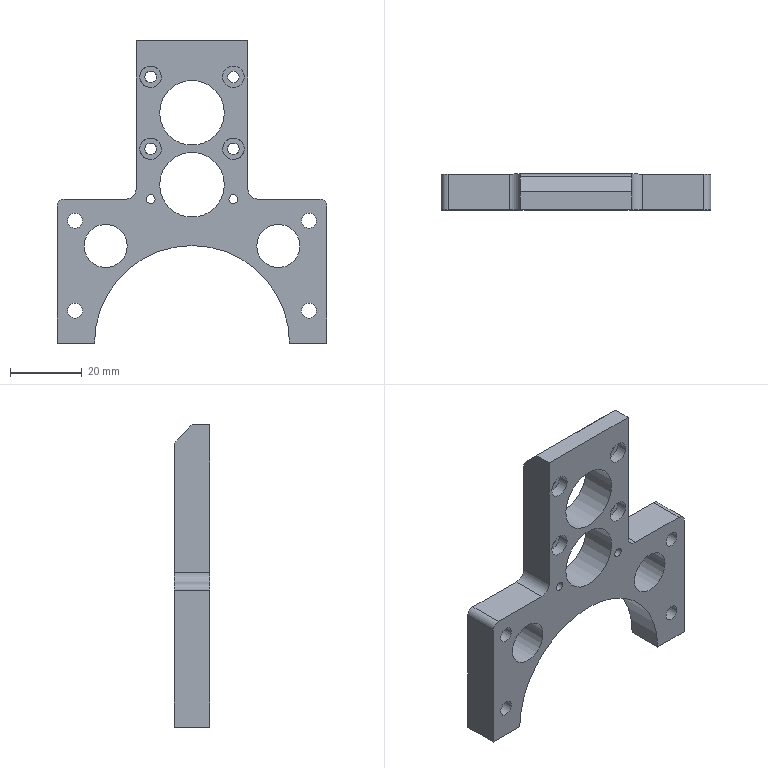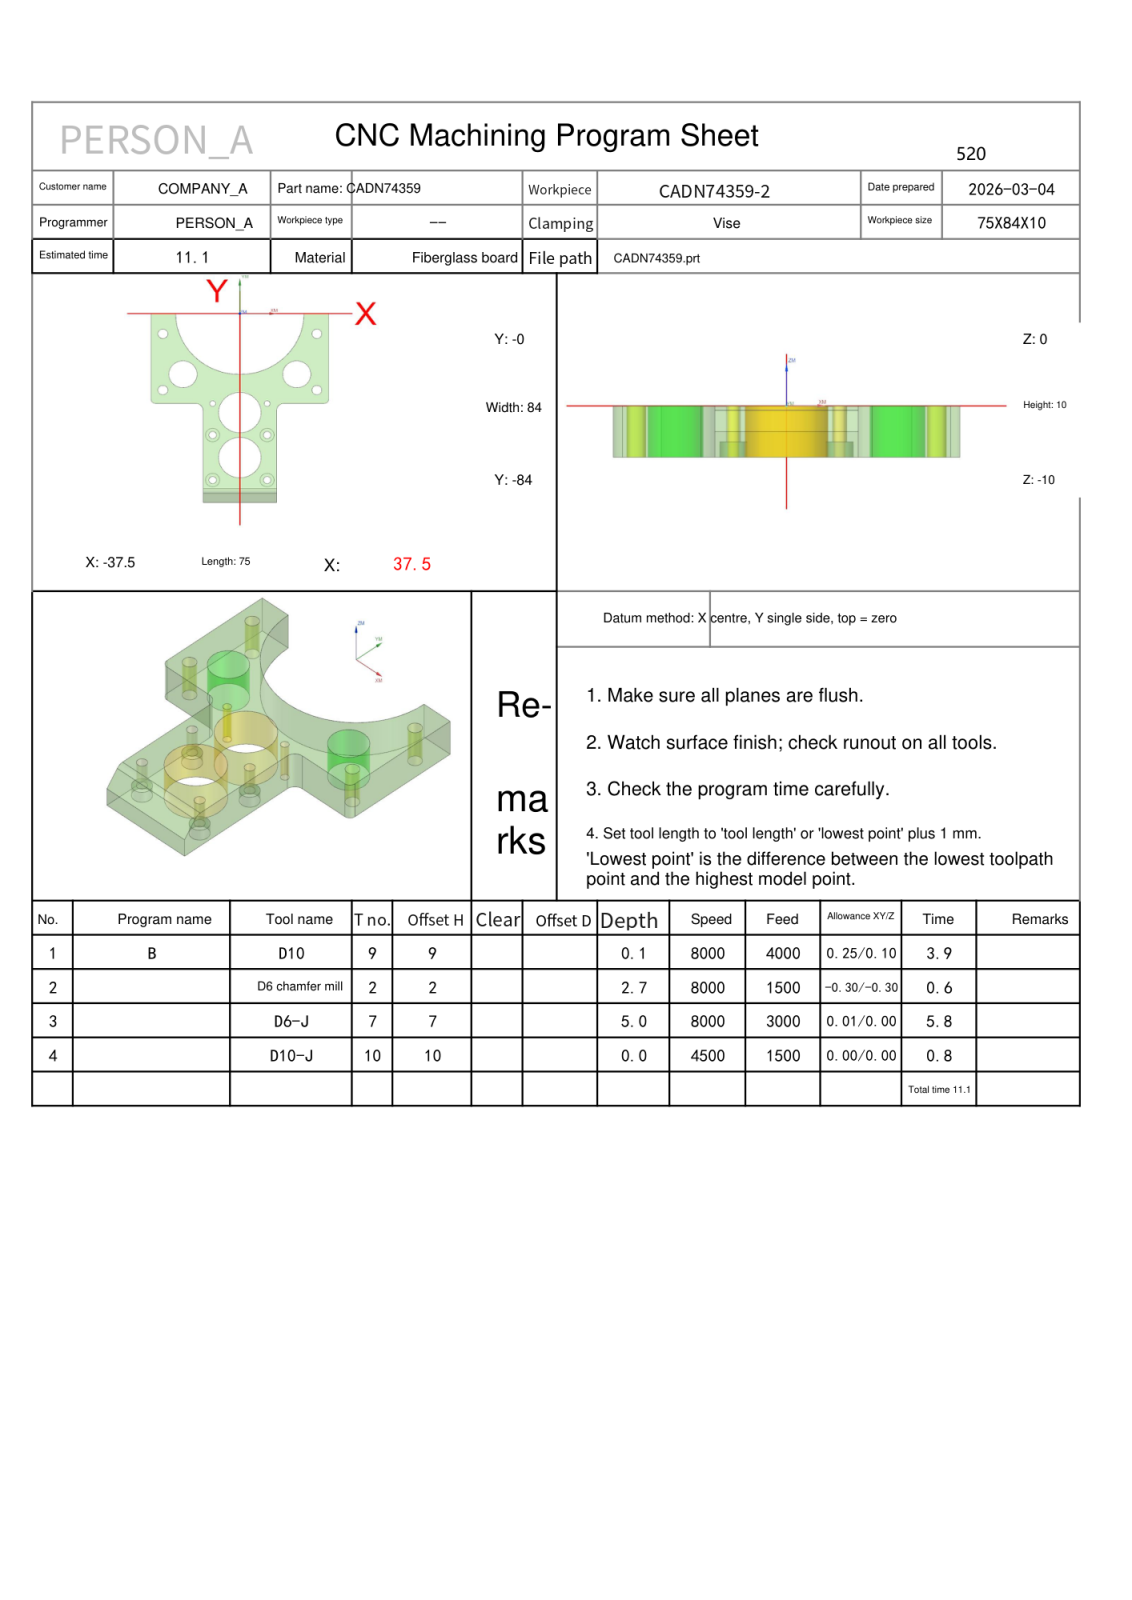NC program | NX | posted by the shop | part box 75 x 10 x 84 mm
Lines 5662 to 5701 of 5701:
N4 T10 M06
(D10-J  D=10. R=0. H=10 ce=0.00 di=0.00)
G00 G90 G54 X-35.962 Y-94. M03 S4500
G43 H10 Z50.
M08
Z2.
G01 Z0.0 F1500.
Y-89.
Y5.
X-29.423
Y-89.
X-22.885
Y5.
X-16.346
Y-89.
X-9.808
Y5.
X-3.269
Y-89.
X3.269
Y5.
X9.808
Y-89.
X16.346
Y5.
X22.885
Y-89.
X29.423
Y5.
X35.962
Y-89.
Y-94.
Z2.
G00 Z50.
M05
M09
G91 G28 Z0.0
G91 G28 Y0.0
M30
%